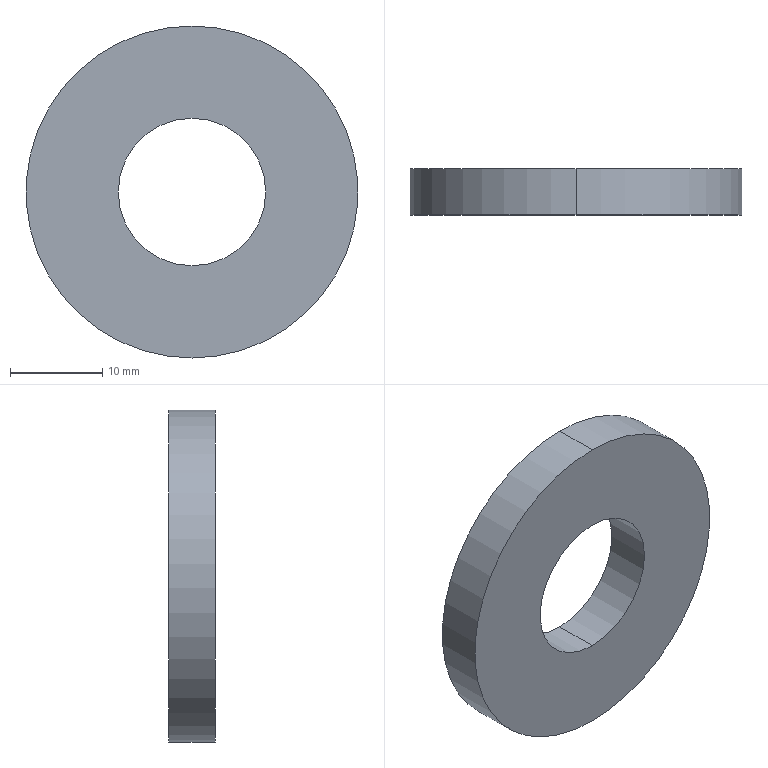Part | SolidWorks | features Extrusion 1 | 1 solid | 6 faces | box 36 x 5 x 36 mm | volume 4084 mm3 | cylinder 4 | plane 2 | commonest cylinder face diameters 16 x2 36 x2
STEP:
#1=CARTESIAN_POINT('',(0.,5.,-8.));
#2=VERTEX_POINT('',#1);
#3=CARTESIAN_POINT('',(0.,5.,8.));
#4=VERTEX_POINT('',#3);
#5=CARTESIAN_POINT('',(0.,5.,0.));
#6=DIRECTION('',(0.,1.,0.));
#7=DIRECTION('',(0.,0.,1.));
#8=AXIS2_PLACEMENT_3D('',#5,#6,#7);
#9=CIRCLE('',#8,8.);
#10=EDGE_CURVE('',#2,#4,#9,.T.);
#11=ORIENTED_EDGE('',*,*,#10,.T.);
#12=CARTESIAN_POINT('',(0.,0.,8.));
#13=VERTEX_POINT('',#12);
#14=CARTESIAN_POINT('',(0.,5.,8.));
#15=DIRECTION('',(0.,-1.,0.));
#16=VECTOR('',#15,1000.);
#17=LINE('',#14,#16);
#18=EDGE_CURVE('',#4,#13,#17,.T.);
#19=ORIENTED_EDGE('',*,*,#18,.T.);
#20=CARTESIAN_POINT('',(0.,0.,-8.));
#21=VERTEX_POINT('',#20);
#22=CARTESIAN_POINT('',(0.,0.,0.));
#23=DIRECTION('',(0.,1.,0.));
#24=DIRECTION('',(0.,0.,1.));
#25=AXIS2_PLACEMENT_3D('',#22,#23,#24);
#26=CIRCLE('',#25,8.);
#27=EDGE_CURVE('',#21,#13,#26,.T.);
#28=ORIENTED_EDGE('',*,*,#27,.F.);
#29=CARTESIAN_POINT('',(0.,5.,-8.));
#30=DIRECTION('',(0.,-1.,0.));
#31=VECTOR('',#30,1000.);
#32=LINE('',#29,#31);
#33=EDGE_CURVE('',#2,#21,#32,.T.);
#34=ORIENTED_EDGE('',*,*,#33,.F.);
#35=EDGE_LOOP('',(#11,#19,#28,#34));
#36=FACE_OUTER_BOUND('',#35,.T.);
#37=CARTESIAN_POINT('',(0.,5.,0.));
#38=DIRECTION('',(0.,-1.,0.));
#39=DIRECTION('',(0.,0.,-1.));
#40=AXIS2_PLACEMENT_3D('',#37,#38,#39);
#41=CYLINDRICAL_SURFACE('',#40,8.);
#42=ADVANCED_FACE('',(#36),#41,.F.);
#43=CARTESIAN_POINT('',(0.,5.,18.));
#44=VERTEX_POINT('',#43);
#45=CARTESIAN_POINT('',(0.,5.,-18.));
#46=VERTEX_POINT('',#45);
#47=CARTESIAN_POINT('',(0.,5.,0.));
#48=DIRECTION('',(0.,1.,0.));
#49=DIRECTION('',(0.,0.,1.));
#50=AXIS2_PLACEMENT_3D('',#47,#48,#49);
#51=CIRCLE('',#50,18.);
#52=EDGE_CURVE('',#44,#46,#51,.T.);
#53=ORIENTED_EDGE('',*,*,#52,.F.);
#54=CARTESIAN_POINT('',(0.,0.,18.));
#55=VERTEX_POINT('',#54);
#56=CARTESIAN_POINT('',(0.,5.,18.));
#57=DIRECTION('',(0.,-1.,0.));
#58=VECTOR('',#57,1000.);
#59=LINE('',#56,#58);
#60=EDGE_CURVE('',#44,#55,#59,.T.);
#61=ORIENTED_EDGE('',*,*,#60,.T.);
#62=CARTESIAN_POINT('',(0.,0.,-18.));
#63=VERTEX_POINT('',#62);
#64=CARTESIAN_POINT('',(0.,0.,0.));
#65=DIRECTION('',(0.,1.,0.));
#66=DIRECTION('',(0.,0.,1.));
#67=AXIS2_PLACEMENT_3D('',#64,#65,#66);
#68=CIRCLE('',#67,18.);
#69=EDGE_CURVE('',#55,#63,#68,.T.);
#70=ORIENTED_EDGE('',*,*,#69,.T.);
#71=CARTESIAN_POINT('',(0.,5.,-18.));
#72=DIRECTION('',(0.,-1.,0.));
#73=VECTOR('',#72,1000.);
#74=LINE('',#71,#73);
#75=EDGE_CURVE('',#46,#63,#74,.T.);
#76=ORIENTED_EDGE('',*,*,#75,.F.);
#77=EDGE_LOOP('',(#53,#61,#70,#76));
#78=FACE_OUTER_BOUND('',#77,.T.);
#79=CARTESIAN_POINT('',(0.,5.,0.));
#80=DIRECTION('',(0.,-1.,0.));
#81=DIRECTION('',(0.,0.,-1.));
#82=AXIS2_PLACEMENT_3D('',#79,#80,#81);
#83=CYLINDRICAL_SURFACE('',#82,18.);
#84=ADVANCED_FACE('',(#78),#83,.T.);
#85=CARTESIAN_POINT('',(0.,5.,0.));
#86=DIRECTION('',(0.,1.,0.));
#87=DIRECTION('',(0.,0.,1.));
#88=AXIS2_PLACEMENT_3D('',#85,#86,#87);
#89=CIRCLE('',#88,18.);
#90=EDGE_CURVE('',#46,#44,#89,.T.);
#91=ORIENTED_EDGE('',*,*,#90,.T.);
#92=ORIENTED_EDGE('',*,*,#52,.T.);
#93=EDGE_LOOP('',(#91,#92));
#94=FACE_OUTER_BOUND('',#93,.T.);
#95=ORIENTED_EDGE('',*,*,#10,.F.);
#96=CARTESIAN_POINT('',(0.,5.,0.));
#97=DIRECTION('',(0.,1.,0.));
#98=DIRECTION('',(0.,0.,1.));
#99=AXIS2_PLACEMENT_3D('',#96,#97,#98);
#100=CIRCLE('',#99,8.);
#101=EDGE_CURVE('',#4,#2,#100,.T.);
#102=ORIENTED_EDGE('',*,*,#101,.F.);
#103=EDGE_LOOP('',(#95,#102));
#104=FACE_BOUND('',#103,.T.);
#105=CARTESIAN_POINT('',(0.,5.,0.));
#106=DIRECTION('',(0.,1.,0.));
#107=DIRECTION('',(0.,0.,1.));
#108=AXIS2_PLACEMENT_3D('',#105,#106,#107);
#109=PLANE('',#108);
#110=ADVANCED_FACE('',(#94,#104),#109,.T.);
#111=CARTESIAN_POINT('',(0.,0.,0.));
#112=DIRECTION('',(0.,1.,0.));
#113=DIRECTION('',(0.,0.,1.));
#114=AXIS2_PLACEMENT_3D('',#111,#112,#113);
#115=CIRCLE('',#114,18.);
#116=EDGE_CURVE('',#63,#55,#115,.T.);
#117=ORIENTED_EDGE('',*,*,#116,.F.);
#118=ORIENTED_EDGE('',*,*,#69,.F.);
#119=EDGE_LOOP('',(#117,#118));
#120=FACE_OUTER_BOUND('',#119,.T.);
#121=ORIENTED_EDGE('',*,*,#27,.T.);
#122=CARTESIAN_POINT('',(0.,0.,0.));
#123=DIRECTION('',(0.,1.,0.));
#124=DIRECTION('',(0.,0.,1.));
#125=AXIS2_PLACEMENT_3D('',#122,#123,#124);
#126=CIRCLE('',#125,8.);
#127=EDGE_CURVE('',#13,#21,#126,.T.);
#128=ORIENTED_EDGE('',*,*,#127,.T.);
#129=EDGE_LOOP('',(#121,#128));
#130=FACE_BOUND('',#129,.T.);
#131=CARTESIAN_POINT('',(0.,0.,0.));
#132=DIRECTION('',(0.,1.,0.));
#133=DIRECTION('',(0.,0.,1.));
#134=AXIS2_PLACEMENT_3D('',#131,#132,#133);
#135=PLANE('',#134);
#136=ADVANCED_FACE('',(#120,#130),#135,.F.);
#137=ORIENTED_EDGE('',*,*,#60,.F.);
#138=ORIENTED_EDGE('',*,*,#90,.F.);
#139=ORIENTED_EDGE('',*,*,#75,.T.);
#140=ORIENTED_EDGE('',*,*,#116,.T.);
#141=EDGE_LOOP('',(#137,#138,#139,#140));
#142=FACE_OUTER_BOUND('',#141,.T.);
#143=CARTESIAN_POINT('',(0.,5.,0.));
#144=DIRECTION('',(0.,-1.,0.));
#145=DIRECTION('',(0.,0.,-1.));
#146=AXIS2_PLACEMENT_3D('',#143,#144,#145);
#147=CYLINDRICAL_SURFACE('',#146,18.);
#148=ADVANCED_FACE('',(#142),#147,.T.);
#149=ORIENTED_EDGE('',*,*,#18,.F.);
#150=ORIENTED_EDGE('',*,*,#101,.T.);
#151=ORIENTED_EDGE('',*,*,#33,.T.);
#152=ORIENTED_EDGE('',*,*,#127,.F.);
#153=EDGE_LOOP('',(#149,#150,#151,#152));
#154=FACE_OUTER_BOUND('',#153,.T.);
#155=CARTESIAN_POINT('',(0.,5.,0.));
#156=DIRECTION('',(0.,-1.,0.));
#157=DIRECTION('',(0.,0.,-1.));
#158=AXIS2_PLACEMENT_3D('',#155,#156,#157);
#159=CYLINDRICAL_SURFACE('',#158,8.);
#160=ADVANCED_FACE('',(#154),#159,.F.);
#161=CLOSED_SHELL('',(#42,#84,#110,#136,#148,#160));
#162=MANIFOLD_SOLID_BREP('',#161);
#163=CARTESIAN_POINT('',(0.,0.,0.));
#164=DIRECTION('',(0.,0.,1.));
#165=DIRECTION('',(1.,0.,0.));
#166=AXIS2_PLACEMENT_3D('',#163,#164,#165);
#167=(LENGTH_UNIT()NAMED_UNIT(*)SI_UNIT(.MILLI.,.METRE.));
#168=UNCERTAINTY_MEASURE_WITH_UNIT(LENGTH_MEASURE(0.00001),#167,'','');
#169=(NAMED_UNIT(*)PLANE_ANGLE_UNIT()SI_UNIT($,.RADIAN.));
#170=(NAMED_UNIT(*)SI_UNIT($,.STERADIAN.)SOLID_ANGLE_UNIT());
#171=(GEOMETRIC_REPRESENTATION_CONTEXT(3)GLOBAL_UNCERTAINTY_ASSIGNED_CONTEXT((#168))GLOBAL_UNIT_ASSIGNED_CONTEXT((#167,#169,#170))REPRESENTATION_CONTEXT('',''));
#172=ADVANCED_BREP_SHAPE_REPRESENTATION('',(#162,#166),#171);